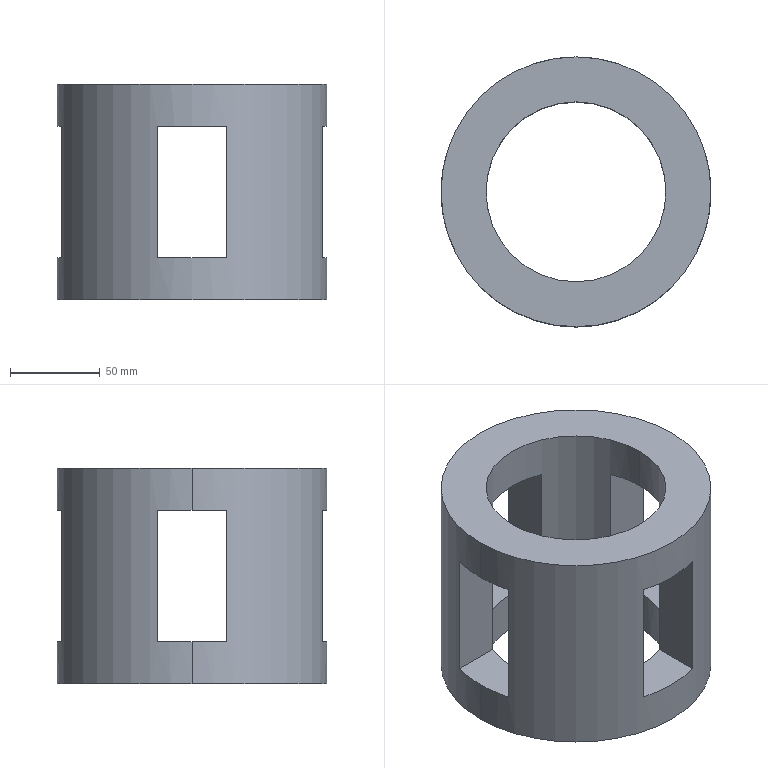Part | SolidWorks | features CirPattern 1, Extrusion 1, ICE 1 | 1 solid | 22 faces | box 150 x 150 x 120 mm | volume 893145 mm3 | plane 18 | cylinder 4 | commonest cylinder face diameters 100 x2 150 x2
STEP:
#1=CARTESIAN_POINT('',(19.196,-46.168,96.484));
#2=VERTEX_POINT('',#1);
#3=CARTESIAN_POINT('',(19.196,-46.168,23.516));
#4=VERTEX_POINT('',#3);
#5=CARTESIAN_POINT('',(19.196,-46.168,120.));
#6=DIRECTION('',(0.,0.,-1.));
#7=VECTOR('',#6,1000.);
#8=LINE('',#5,#7);
#9=EDGE_CURVE('',#2,#4,#8,.T.);
#10=ORIENTED_EDGE('',*,*,#9,.F.);
#11=CARTESIAN_POINT('',(-19.196,-46.168,96.484));
#12=VERTEX_POINT('',#11);
#13=CARTESIAN_POINT('',(0.,0.,96.484));
#14=DIRECTION('',(0.,0.,1.));
#15=DIRECTION('',(1.,0.,0.));
#16=AXIS2_PLACEMENT_3D('',#13,#14,#15);
#17=CIRCLE('',#16,50.);
#18=EDGE_CURVE('',#12,#2,#17,.T.);
#19=ORIENTED_EDGE('',*,*,#18,.F.);
#20=CARTESIAN_POINT('',(-19.196,-46.168,23.516));
#21=VERTEX_POINT('',#20);
#22=CARTESIAN_POINT('',(-19.196,-46.168,120.));
#23=DIRECTION('',(0.,0.,1.));
#24=VECTOR('',#23,1000.);
#25=LINE('',#22,#24);
#26=EDGE_CURVE('',#21,#12,#25,.T.);
#27=ORIENTED_EDGE('',*,*,#26,.F.);
#28=CARTESIAN_POINT('',(0.,0.,23.516));
#29=DIRECTION('',(0.,0.,-1.));
#30=DIRECTION('',(-1.,0.,0.));
#31=AXIS2_PLACEMENT_3D('',#28,#29,#30);
#32=CIRCLE('',#31,50.);
#33=EDGE_CURVE('',#4,#21,#32,.T.);
#34=ORIENTED_EDGE('',*,*,#33,.F.);
#35=EDGE_LOOP('',(#10,#19,#27,#34));
#36=FACE_BOUND('',#35,.T.);
#37=CARTESIAN_POINT('',(-50.,0.,120.));
#38=VERTEX_POINT('',#37);
#39=CARTESIAN_POINT('',(50.,0.,120.));
#40=VERTEX_POINT('',#39);
#41=CARTESIAN_POINT('',(0.,0.,120.));
#42=DIRECTION('',(0.,0.,1.));
#43=DIRECTION('',(1.,0.,0.));
#44=AXIS2_PLACEMENT_3D('',#41,#42,#43);
#45=CIRCLE('',#44,50.);
#46=EDGE_CURVE('',#38,#40,#45,.T.);
#47=ORIENTED_EDGE('',*,*,#46,.T.);
#48=CARTESIAN_POINT('',(50.,0.,96.484));
#49=VERTEX_POINT('',#48);
#50=CARTESIAN_POINT('',(50.,0.,120.));
#51=DIRECTION('',(0.,0.,-1.));
#52=VECTOR('',#51,1000.);
#53=LINE('',#50,#52);
#54=EDGE_CURVE('',#40,#49,#53,.T.);
#55=ORIENTED_EDGE('',*,*,#54,.T.);
#56=CARTESIAN_POINT('',(46.168,-19.196,96.484));
#57=VERTEX_POINT('',#56);
#58=CARTESIAN_POINT('',(0.,0.,96.484));
#59=DIRECTION('',(0.,0.,1.));
#60=DIRECTION('',(1.,0.,0.));
#61=AXIS2_PLACEMENT_3D('',#58,#59,#60);
#62=CIRCLE('',#61,50.);
#63=EDGE_CURVE('',#57,#49,#62,.T.);
#64=ORIENTED_EDGE('',*,*,#63,.F.);
#65=CARTESIAN_POINT('',(46.168,-19.196,23.516));
#66=VERTEX_POINT('',#65);
#67=CARTESIAN_POINT('',(46.168,-19.196,120.));
#68=DIRECTION('',(0.,0.,1.));
#69=VECTOR('',#68,1000.);
#70=LINE('',#67,#69);
#71=EDGE_CURVE('',#66,#57,#70,.T.);
#72=ORIENTED_EDGE('',*,*,#71,.F.);
#73=CARTESIAN_POINT('',(50.,0.,23.516));
#74=VERTEX_POINT('',#73);
#75=CARTESIAN_POINT('',(0.,0.,23.516));
#76=DIRECTION('',(0.,0.,-1.));
#77=DIRECTION('',(-1.,0.,0.));
#78=AXIS2_PLACEMENT_3D('',#75,#76,#77);
#79=CIRCLE('',#78,50.);
#80=EDGE_CURVE('',#74,#66,#79,.T.);
#81=ORIENTED_EDGE('',*,*,#80,.F.);
#82=CARTESIAN_POINT('',(50.,0.,0.));
#83=VERTEX_POINT('',#82);
#84=CARTESIAN_POINT('',(50.,0.,120.));
#85=DIRECTION('',(0.,0.,-1.));
#86=VECTOR('',#85,1000.);
#87=LINE('',#84,#86);
#88=EDGE_CURVE('',#74,#83,#87,.T.);
#89=ORIENTED_EDGE('',*,*,#88,.T.);
#90=CARTESIAN_POINT('',(-50.,0.,0.));
#91=VERTEX_POINT('',#90);
#92=CARTESIAN_POINT('',(0.,0.,0.));
#93=DIRECTION('',(0.,0.,1.));
#94=DIRECTION('',(1.,0.,0.));
#95=AXIS2_PLACEMENT_3D('',#92,#93,#94);
#96=CIRCLE('',#95,50.);
#97=EDGE_CURVE('',#91,#83,#96,.T.);
#98=ORIENTED_EDGE('',*,*,#97,.F.);
#99=CARTESIAN_POINT('',(-50.,0.,23.516));
#100=VERTEX_POINT('',#99);
#101=CARTESIAN_POINT('',(-50.,0.,120.));
#102=DIRECTION('',(0.,0.,-1.));
#103=VECTOR('',#102,1000.);
#104=LINE('',#101,#103);
#105=EDGE_CURVE('',#100,#91,#104,.T.);
#106=ORIENTED_EDGE('',*,*,#105,.F.);
#107=CARTESIAN_POINT('',(-46.168,-19.196,23.516));
#108=VERTEX_POINT('',#107);
#109=CARTESIAN_POINT('',(0.,0.,23.516));
#110=DIRECTION('',(0.,0.,-1.));
#111=DIRECTION('',(-1.,0.,0.));
#112=AXIS2_PLACEMENT_3D('',#109,#110,#111);
#113=CIRCLE('',#112,50.);
#114=EDGE_CURVE('',#108,#100,#113,.T.);
#115=ORIENTED_EDGE('',*,*,#114,.F.);
#116=CARTESIAN_POINT('',(-46.168,-19.196,96.484));
#117=VERTEX_POINT('',#116);
#118=CARTESIAN_POINT('',(-46.168,-19.196,120.));
#119=DIRECTION('',(0.,0.,-1.));
#120=VECTOR('',#119,1000.);
#121=LINE('',#118,#120);
#122=EDGE_CURVE('',#117,#108,#121,.T.);
#123=ORIENTED_EDGE('',*,*,#122,.F.);
#124=CARTESIAN_POINT('',(-50.,0.,96.484));
#125=VERTEX_POINT('',#124);
#126=CARTESIAN_POINT('',(0.,0.,96.484));
#127=DIRECTION('',(0.,0.,1.));
#128=DIRECTION('',(1.,0.,0.));
#129=AXIS2_PLACEMENT_3D('',#126,#127,#128);
#130=CIRCLE('',#129,50.);
#131=EDGE_CURVE('',#125,#117,#130,.T.);
#132=ORIENTED_EDGE('',*,*,#131,.F.);
#133=CARTESIAN_POINT('',(-50.,0.,120.));
#134=DIRECTION('',(0.,0.,-1.));
#135=VECTOR('',#134,1000.);
#136=LINE('',#133,#135);
#137=EDGE_CURVE('',#38,#125,#136,.T.);
#138=ORIENTED_EDGE('',*,*,#137,.F.);
#139=EDGE_LOOP('',(#47,#55,#64,#72,#81,#89,#98,#106,#115,#123,#132,#138));
#140=FACE_OUTER_BOUND('',#139,.T.);
#141=CARTESIAN_POINT('',(0.,0.,120.));
#142=DIRECTION('',(0.,0.,-1.));
#143=DIRECTION('',(-1.,0.,0.));
#144=AXIS2_PLACEMENT_3D('',#141,#142,#143);
#145=CYLINDRICAL_SURFACE('',#144,50.);
#146=ADVANCED_FACE('',(#36,#140),#145,.F.);
#147=CARTESIAN_POINT('',(19.196,72.502,23.516));
#148=VERTEX_POINT('',#147);
#149=CARTESIAN_POINT('',(19.196,72.502,96.484));
#150=VERTEX_POINT('',#149);
#151=CARTESIAN_POINT('',(19.196,72.502,120.));
#152=DIRECTION('',(0.,0.,1.));
#153=VECTOR('',#152,1000.);
#154=LINE('',#151,#153);
#155=EDGE_CURVE('',#148,#150,#154,.T.);
#156=ORIENTED_EDGE('',*,*,#155,.T.);
#157=CARTESIAN_POINT('',(-19.196,72.502,96.484));
#158=VERTEX_POINT('',#157);
#159=CARTESIAN_POINT('',(0.,0.,96.484));
#160=DIRECTION('',(0.,0.,1.));
#161=DIRECTION('',(1.,0.,0.));
#162=AXIS2_PLACEMENT_3D('',#159,#160,#161);
#163=CIRCLE('',#162,75.);
#164=EDGE_CURVE('',#150,#158,#163,.T.);
#165=ORIENTED_EDGE('',*,*,#164,.T.);
#166=CARTESIAN_POINT('',(-19.196,72.502,23.516));
#167=VERTEX_POINT('',#166);
#168=CARTESIAN_POINT('',(-19.196,72.502,120.));
#169=DIRECTION('',(0.,0.,-1.));
#170=VECTOR('',#169,1000.);
#171=LINE('',#168,#170);
#172=EDGE_CURVE('',#158,#167,#171,.T.);
#173=ORIENTED_EDGE('',*,*,#172,.T.);
#174=CARTESIAN_POINT('',(0.,0.,23.516));
#175=DIRECTION('',(0.,0.,-1.));
#176=DIRECTION('',(-1.,0.,0.));
#177=AXIS2_PLACEMENT_3D('',#174,#175,#176);
#178=CIRCLE('',#177,75.);
#179=EDGE_CURVE('',#167,#148,#178,.T.);
#180=ORIENTED_EDGE('',*,*,#179,.T.);
#181=EDGE_LOOP('',(#156,#165,#173,#180));
#182=FACE_BOUND('',#181,.T.);
#183=CARTESIAN_POINT('',(75.,0.,120.));
#184=VERTEX_POINT('',#183);
#185=CARTESIAN_POINT('',(-75.,0.,120.));
#186=VERTEX_POINT('',#185);
#187=CARTESIAN_POINT('',(0.,0.,120.));
#188=DIRECTION('',(0.,0.,1.));
#189=DIRECTION('',(1.,0.,0.));
#190=AXIS2_PLACEMENT_3D('',#187,#188,#189);
#191=CIRCLE('',#190,75.);
#192=EDGE_CURVE('',#184,#186,#191,.T.);
#193=ORIENTED_EDGE('',*,*,#192,.F.);
#194=CARTESIAN_POINT('',(75.,0.,96.484));
#195=VERTEX_POINT('',#194);
#196=CARTESIAN_POINT('',(75.,0.,120.));
#197=DIRECTION('',(0.,0.,-1.));
#198=VECTOR('',#197,1000.);
#199=LINE('',#196,#198);
#200=EDGE_CURVE('',#184,#195,#199,.T.);
#201=ORIENTED_EDGE('',*,*,#200,.T.);
#202=CARTESIAN_POINT('',(72.502,19.196,96.484));
#203=VERTEX_POINT('',#202);
#204=CARTESIAN_POINT('',(0.,0.,96.484));
#205=DIRECTION('',(0.,0.,1.));
#206=DIRECTION('',(1.,0.,0.));
#207=AXIS2_PLACEMENT_3D('',#204,#205,#206);
#208=CIRCLE('',#207,75.);
#209=EDGE_CURVE('',#195,#203,#208,.T.);
#210=ORIENTED_EDGE('',*,*,#209,.T.);
#211=CARTESIAN_POINT('',(72.502,19.196,23.516));
#212=VERTEX_POINT('',#211);
#213=CARTESIAN_POINT('',(72.502,19.196,120.));
#214=DIRECTION('',(0.,0.,-1.));
#215=VECTOR('',#214,1000.);
#216=LINE('',#213,#215);
#217=EDGE_CURVE('',#203,#212,#216,.T.);
#218=ORIENTED_EDGE('',*,*,#217,.T.);
#219=CARTESIAN_POINT('',(75.,0.,23.516));
#220=VERTEX_POINT('',#219);
#221=CARTESIAN_POINT('',(0.,0.,23.516));
#222=DIRECTION('',(0.,0.,-1.));
#223=DIRECTION('',(-1.,0.,0.));
#224=AXIS2_PLACEMENT_3D('',#221,#222,#223);
#225=CIRCLE('',#224,75.);
#226=EDGE_CURVE('',#212,#220,#225,.T.);
#227=ORIENTED_EDGE('',*,*,#226,.T.);
#228=CARTESIAN_POINT('',(75.,0.,0.));
#229=VERTEX_POINT('',#228);
#230=CARTESIAN_POINT('',(75.,0.,120.));
#231=DIRECTION('',(0.,0.,-1.));
#232=VECTOR('',#231,1000.);
#233=LINE('',#230,#232);
#234=EDGE_CURVE('',#220,#229,#233,.T.);
#235=ORIENTED_EDGE('',*,*,#234,.T.);
#236=CARTESIAN_POINT('',(-75.,0.,0.));
#237=VERTEX_POINT('',#236);
#238=CARTESIAN_POINT('',(0.,0.,0.));
#239=DIRECTION('',(0.,0.,1.));
#240=DIRECTION('',(1.,0.,0.));
#241=AXIS2_PLACEMENT_3D('',#238,#239,#240);
#242=CIRCLE('',#241,75.);
#243=EDGE_CURVE('',#229,#237,#242,.T.);
#244=ORIENTED_EDGE('',*,*,#243,.T.);
#245=CARTESIAN_POINT('',(-75.,0.,23.516));
#246=VERTEX_POINT('',#245);
#247=CARTESIAN_POINT('',(-75.,0.,120.));
#248=DIRECTION('',(0.,0.,-1.));
#249=VECTOR('',#248,1000.);
#250=LINE('',#247,#249);
#251=EDGE_CURVE('',#246,#237,#250,.T.);
#252=ORIENTED_EDGE('',*,*,#251,.F.);
#253=CARTESIAN_POINT('',(-72.502,19.196,23.516));
#254=VERTEX_POINT('',#253);
#255=CARTESIAN_POINT('',(0.,0.,23.516));
#256=DIRECTION('',(0.,0.,-1.));
#257=DIRECTION('',(-1.,0.,0.));
#258=AXIS2_PLACEMENT_3D('',#255,#256,#257);
#259=CIRCLE('',#258,75.);
#260=EDGE_CURVE('',#246,#254,#259,.T.);
#261=ORIENTED_EDGE('',*,*,#260,.T.);
#262=CARTESIAN_POINT('',(-72.502,19.196,96.484));
#263=VERTEX_POINT('',#262);
#264=CARTESIAN_POINT('',(-72.502,19.196,120.));
#265=DIRECTION('',(0.,0.,1.));
#266=VECTOR('',#265,1000.);
#267=LINE('',#264,#266);
#268=EDGE_CURVE('',#254,#263,#267,.T.);
#269=ORIENTED_EDGE('',*,*,#268,.T.);
#270=CARTESIAN_POINT('',(-75.,0.,96.484));
#271=VERTEX_POINT('',#270);
#272=CARTESIAN_POINT('',(0.,0.,96.484));
#273=DIRECTION('',(0.,0.,1.));
#274=DIRECTION('',(1.,0.,0.));
#275=AXIS2_PLACEMENT_3D('',#272,#273,#274);
#276=CIRCLE('',#275,75.);
#277=EDGE_CURVE('',#263,#271,#276,.T.);
#278=ORIENTED_EDGE('',*,*,#277,.T.);
#279=CARTESIAN_POINT('',(-75.,0.,120.));
#280=DIRECTION('',(0.,0.,-1.));
#281=VECTOR('',#280,1000.);
#282=LINE('',#279,#281);
#283=EDGE_CURVE('',#186,#271,#282,.T.);
#284=ORIENTED_EDGE('',*,*,#283,.F.);
#285=EDGE_LOOP('',(#193,#201,#210,#218,#227,#235,#244,#252,#261,#269,#278,#284));
#286=FACE_OUTER_BOUND('',#285,.T.);
#287=CARTESIAN_POINT('',(0.,0.,120.));
#288=DIRECTION('',(0.,0.,-1.));
#289=DIRECTION('',(-1.,0.,0.));
#290=AXIS2_PLACEMENT_3D('',#287,#288,#289);
#291=CYLINDRICAL_SURFACE('',#290,75.);
#292=ADVANCED_FACE('',(#182,#286),#291,.T.);
#293=CARTESIAN_POINT('',(0.,0.,120.));
#294=DIRECTION('',(0.,0.,1.));
#295=DIRECTION('',(1.,0.,0.));
#296=AXIS2_PLACEMENT_3D('',#293,#294,#295);
#297=CIRCLE('',#296,75.);
#298=EDGE_CURVE('',#186,#184,#297,.T.);
#299=ORIENTED_EDGE('',*,*,#298,.T.);
#300=ORIENTED_EDGE('',*,*,#192,.T.);
#301=EDGE_LOOP('',(#299,#300));
#302=FACE_OUTER_BOUND('',#301,.T.);
#303=ORIENTED_EDGE('',*,*,#46,.F.);
#304=CARTESIAN_POINT('',(0.,0.,120.));
#305=DIRECTION('',(0.,0.,1.));
#306=DIRECTION('',(1.,0.,0.));
#307=AXIS2_PLACEMENT_3D('',#304,#305,#306);
#308=CIRCLE('',#307,50.);
#309=EDGE_CURVE('',#40,#38,#308,.T.);
#310=ORIENTED_EDGE('',*,*,#309,.F.);
#311=EDGE_LOOP('',(#303,#310));
#312=FACE_BOUND('',#311,.T.);
#313=CARTESIAN_POINT('',(0.,0.,120.));
#314=DIRECTION('',(0.,0.,1.));
#315=DIRECTION('',(1.,0.,0.));
#316=AXIS2_PLACEMENT_3D('',#313,#314,#315);
#317=PLANE('',#316);
#318=ADVANCED_FACE('',(#302,#312),#317,.T.);
#319=CARTESIAN_POINT('',(0.,0.,0.));
#320=DIRECTION('',(0.,0.,1.));
#321=DIRECTION('',(1.,0.,0.));
#322=AXIS2_PLACEMENT_3D('',#319,#320,#321);
#323=CIRCLE('',#322,75.);
#324=EDGE_CURVE('',#237,#229,#323,.T.);
#325=ORIENTED_EDGE('',*,*,#324,.F.);
#326=ORIENTED_EDGE('',*,*,#243,.F.);
#327=EDGE_LOOP('',(#325,#326));
#328=FACE_OUTER_BOUND('',#327,.T.);
#329=ORIENTED_EDGE('',*,*,#97,.T.);
#330=CARTESIAN_POINT('',(0.,0.,0.));
#331=DIRECTION('',(0.,0.,1.));
#332=DIRECTION('',(1.,0.,0.));
#333=AXIS2_PLACEMENT_3D('',#330,#331,#332);
#334=CIRCLE('',#333,50.);
#335=EDGE_CURVE('',#83,#91,#334,.T.);
#336=ORIENTED_EDGE('',*,*,#335,.T.);
#337=EDGE_LOOP('',(#329,#336));
#338=FACE_BOUND('',#337,.T.);
#339=CARTESIAN_POINT('',(0.,0.,0.));
#340=DIRECTION('',(0.,0.,1.));
#341=DIRECTION('',(1.,0.,0.));
#342=AXIS2_PLACEMENT_3D('',#339,#340,#341);
#343=PLANE('',#342);
#344=ADVANCED_FACE('',(#328,#338),#343,.F.);
#345=ORIENTED_EDGE('',*,*,#200,.F.);
#346=ORIENTED_EDGE('',*,*,#298,.F.);
#347=ORIENTED_EDGE('',*,*,#283,.T.);
#348=CARTESIAN_POINT('',(-72.502,-19.196,96.484));
#349=VERTEX_POINT('',#348);
#350=CARTESIAN_POINT('',(0.,0.,96.484));
#351=DIRECTION('',(0.,0.,1.));
#352=DIRECTION('',(1.,0.,0.));
#353=AXIS2_PLACEMENT_3D('',#350,#351,#352);
#354=CIRCLE('',#353,75.);
#355=EDGE_CURVE('',#271,#349,#354,.T.);
#356=ORIENTED_EDGE('',*,*,#355,.T.);
#357=CARTESIAN_POINT('',(-72.502,-19.196,23.516));
#358=VERTEX_POINT('',#357);
#359=CARTESIAN_POINT('',(-72.502,-19.196,120.));
#360=DIRECTION('',(0.,0.,-1.));
#361=VECTOR('',#360,1000.);
#362=LINE('',#359,#361);
#363=EDGE_CURVE('',#349,#358,#362,.T.);
#364=ORIENTED_EDGE('',*,*,#363,.T.);
#365=CARTESIAN_POINT('',(0.,0.,23.516));
#366=DIRECTION('',(0.,0.,-1.));
#367=DIRECTION('',(-1.,0.,0.));
#368=AXIS2_PLACEMENT_3D('',#365,#366,#367);
#369=CIRCLE('',#368,75.);
#370=EDGE_CURVE('',#358,#246,#369,.T.);
#371=ORIENTED_EDGE('',*,*,#370,.T.);
#372=ORIENTED_EDGE('',*,*,#251,.T.);
#373=ORIENTED_EDGE('',*,*,#324,.T.);
#374=ORIENTED_EDGE('',*,*,#234,.F.);
#375=CARTESIAN_POINT('',(72.502,-19.196,23.516));
#376=VERTEX_POINT('',#375);
#377=CARTESIAN_POINT('',(0.,0.,23.516));
#378=DIRECTION('',(0.,0.,-1.));
#379=DIRECTION('',(-1.,0.,0.));
#380=AXIS2_PLACEMENT_3D('',#377,#378,#379);
#381=CIRCLE('',#380,75.);
#382=EDGE_CURVE('',#220,#376,#381,.T.);
#383=ORIENTED_EDGE('',*,*,#382,.T.);
#384=CARTESIAN_POINT('',(72.502,-19.196,96.484));
#385=VERTEX_POINT('',#384);
#386=CARTESIAN_POINT('',(72.502,-19.196,120.));
#387=DIRECTION('',(0.,0.,1.));
#388=VECTOR('',#387,1000.);
#389=LINE('',#386,#388);
#390=EDGE_CURVE('',#376,#385,#389,.T.);
#391=ORIENTED_EDGE('',*,*,#390,.T.);
#392=CARTESIAN_POINT('',(0.,0.,96.484));
#393=DIRECTION('',(0.,0.,1.));
#394=DIRECTION('',(1.,0.,0.));
#395=AXIS2_PLACEMENT_3D('',#392,#393,#394);
#396=CIRCLE('',#395,75.);
#397=EDGE_CURVE('',#385,#195,#396,.T.);
#398=ORIENTED_EDGE('',*,*,#397,.T.);
#399=EDGE_LOOP('',(#345,#346,#347,#356,#364,#371,#372,#373,#374,#383,#391,#398));
#400=FACE_OUTER_BOUND('',#399,.T.);
#401=CARTESIAN_POINT('',(19.196,-72.502,96.484));
#402=VERTEX_POINT('',#401);
#403=CARTESIAN_POINT('',(19.196,-72.502,23.516));
#404=VERTEX_POINT('',#403);
#405=CARTESIAN_POINT('',(19.196,-72.502,120.));
#406=DIRECTION('',(0.,0.,-1.));
#407=VECTOR('',#406,1000.);
#408=LINE('',#405,#407);
#409=EDGE_CURVE('',#402,#404,#408,.T.);
#410=ORIENTED_EDGE('',*,*,#409,.T.);
#411=CARTESIAN_POINT('',(-19.196,-72.502,23.516));
#412=VERTEX_POINT('',#411);
#413=CARTESIAN_POINT('',(0.,0.,23.516));
#414=DIRECTION('',(0.,0.,-1.));
#415=DIRECTION('',(-1.,0.,0.));
#416=AXIS2_PLACEMENT_3D('',#413,#414,#415);
#417=CIRCLE('',#416,75.);
#418=EDGE_CURVE('',#404,#412,#417,.T.);
#419=ORIENTED_EDGE('',*,*,#418,.T.);
#420=CARTESIAN_POINT('',(-19.196,-72.502,96.484));
#421=VERTEX_POINT('',#420);
#422=CARTESIAN_POINT('',(-19.196,-72.502,120.));
#423=DIRECTION('',(0.,0.,1.));
#424=VECTOR('',#423,1000.);
#425=LINE('',#422,#424);
#426=EDGE_CURVE('',#412,#421,#425,.T.);
#427=ORIENTED_EDGE('',*,*,#426,.T.);
#428=CARTESIAN_POINT('',(0.,0.,96.484));
#429=DIRECTION('',(0.,0.,1.));
#430=DIRECTION('',(1.,0.,0.));
#431=AXIS2_PLACEMENT_3D('',#428,#429,#430);
#432=CIRCLE('',#431,75.);
#433=EDGE_CURVE('',#421,#402,#432,.T.);
#434=ORIENTED_EDGE('',*,*,#433,.T.);
#435=EDGE_LOOP('',(#410,#419,#427,#434));
#436=FACE_BOUND('',#435,.T.);
#437=CARTESIAN_POINT('',(0.,0.,120.));
#438=DIRECTION('',(0.,0.,-1.));
#439=DIRECTION('',(-1.,0.,0.));
#440=AXIS2_PLACEMENT_3D('',#437,#438,#439);
#441=CYLINDRICAL_SURFACE('',#440,75.);
#442=ADVANCED_FACE('',(#400,#436),#441,.T.);
#443=ORIENTED_EDGE('',*,*,#54,.F.);
#444=ORIENTED_EDGE('',*,*,#309,.T.);
#445=ORIENTED_EDGE('',*,*,#137,.T.);
#446=CARTESIAN_POINT('',(-46.168,19.196,96.484));
#447=VERTEX_POINT('',#446);
#448=CARTESIAN_POINT('',(0.,0.,96.484));
#449=DIRECTION('',(0.,0.,1.));
#450=DIRECTION('',(1.,0.,0.));
#451=AXIS2_PLACEMENT_3D('',#448,#449,#450);
#452=CIRCLE('',#451,50.);
#453=EDGE_CURVE('',#447,#125,#452,.T.);
#454=ORIENTED_EDGE('',*,*,#453,.F.);
#455=CARTESIAN_POINT('',(-46.168,19.196,23.516));
#456=VERTEX_POINT('',#455);
#457=CARTESIAN_POINT('',(-46.168,19.196,120.));
#458=DIRECTION('',(0.,0.,1.));
#459=VECTOR('',#458,1000.);
#460=LINE('',#457,#459);
#461=EDGE_CURVE('',#456,#447,#460,.T.);
#462=ORIENTED_EDGE('',*,*,#461,.F.);
#463=CARTESIAN_POINT('',(0.,0.,23.516));
#464=DIRECTION('',(0.,0.,-1.));
#465=DIRECTION('',(-1.,0.,0.));
#466=AXIS2_PLACEMENT_3D('',#463,#464,#465);
#467=CIRCLE('',#466,50.);
#468=EDGE_CURVE('',#100,#456,#467,.T.);
#469=ORIENTED_EDGE('',*,*,#468,.F.);
#470=ORIENTED_EDGE('',*,*,#105,.T.);
#471=ORIENTED_EDGE('',*,*,#335,.F.);
#472=ORIENTED_EDGE('',*,*,#88,.F.);
#473=CARTESIAN_POINT('',(46.168,19.196,23.516));
#474=VERTEX_POINT('',#473);
#475=CARTESIAN_POINT('',(0.,0.,23.516));
#476=DIRECTION('',(0.,0.,-1.));
#477=DIRECTION('',(-1.,0.,0.));
#478=AXIS2_PLACEMENT_3D('',#475,#476,#477);
#479=CIRCLE('',#478,50.);
#480=EDGE_CURVE('',#474,#74,#479,.T.);
#481=ORIENTED_EDGE('',*,*,#480,.F.);
#482=CARTESIAN_POINT('',(46.168,19.196,96.484));
#483=VERTEX_POINT('',#482);
#484=CARTESIAN_POINT('',(46.168,19.196,120.));
#485=DIRECTION('',(0.,0.,-1.));
#486=VECTOR('',#485,1000.);
#487=LINE('',#484,#486);
#488=EDGE_CURVE('',#483,#474,#487,.T.);
#489=ORIENTED_EDGE('',*,*,#488,.F.);
#490=CARTESIAN_POINT('',(0.,0.,96.484));
#491=DIRECTION('',(0.,0.,1.));
#492=DIRECTION('',(1.,0.,0.));
#493=AXIS2_PLACEMENT_3D('',#490,#491,#492);
#494=CIRCLE('',#493,50.);
#495=EDGE_CURVE('',#49,#483,#494,.T.);
#496=ORIENTED_EDGE('',*,*,#495,.F.);
#497=EDGE_LOOP('',(#443,#444,#445,#454,#462,#469,#470,#471,#472,#481,#489,#496));
#498=FACE_OUTER_BOUND('',#497,.T.);
#499=CARTESIAN_POINT('',(-19.196,46.168,96.484));
#500=VERTEX_POINT('',#499);
#501=CARTESIAN_POINT('',(-19.196,46.168,23.516));
#502=VERTEX_POINT('',#501);
#503=CARTESIAN_POINT('',(-19.196,46.168,120.));
#504=DIRECTION('',(0.,0.,-1.));
#505=VECTOR('',#504,1000.);
#506=LINE('',#503,#505);
#507=EDGE_CURVE('',#500,#502,#506,.T.);
#508=ORIENTED_EDGE('',*,*,#507,.F.);
#509=CARTESIAN_POINT('',(19.196,46.168,96.484));
#510=VERTEX_POINT('',#509);
#511=CARTESIAN_POINT('',(0.,0.,96.484));
#512=DIRECTION('',(0.,0.,1.));
#513=DIRECTION('',(1.,0.,0.));
#514=AXIS2_PLACEMENT_3D('',#511,#512,#513);
#515=CIRCLE('',#514,50.);
#516=EDGE_CURVE('',#510,#500,#515,.T.);
#517=ORIENTED_EDGE('',*,*,#516,.F.);
#518=CARTESIAN_POINT('',(19.196,46.168,23.516));
#519=VERTEX_POINT('',#518);
#520=CARTESIAN_POINT('',(19.196,46.168,120.));
#521=DIRECTION('',(0.,0.,1.));
#522=VECTOR('',#521,1000.);
#523=LINE('',#520,#522);
#524=EDGE_CURVE('',#519,#510,#523,.T.);
#525=ORIENTED_EDGE('',*,*,#524,.F.);
#526=CARTESIAN_POINT('',(0.,0.,23.516));
#527=DIRECTION('',(0.,0.,-1.));
#528=DIRECTION('',(-1.,0.,0.));
#529=AXIS2_PLACEMENT_3D('',#526,#527,#528);
#530=CIRCLE('',#529,50.);
#531=EDGE_CURVE('',#502,#519,#530,.T.);
#532=ORIENTED_EDGE('',*,*,#531,.F.);
#533=EDGE_LOOP('',(#508,#517,#525,#532));
#534=FACE_BOUND('',#533,.T.);
#535=CARTESIAN_POINT('',(0.,0.,120.));
#536=DIRECTION('',(0.,0.,-1.));
#537=DIRECTION('',(-1.,0.,0.));
#538=AXIS2_PLACEMENT_3D('',#535,#536,#537);
#539=CYLINDRICAL_SURFACE('',#538,50.);
#540=ADVANCED_FACE('',(#498,#534),#539,.F.);
#541=CARTESIAN_POINT('',(19.196,-75.,96.484));
#542=DIRECTION('',(0.,1.,0.));
#543=VECTOR('',#542,1000.);
#544=LINE('',#541,#543);
#545=EDGE_CURVE('',#402,#2,#544,.T.);
#546=ORIENTED_EDGE('',*,*,#545,.T.);
#547=ORIENTED_EDGE('',*,*,#9,.T.);
#548=CARTESIAN_POINT('',(19.196,-75.,23.516));
#549=DIRECTION('',(0.,1.,0.));
#550=VECTOR('',#549,1000.);
#551=LINE('',#548,#550);
#552=EDGE_CURVE('',#404,#4,#551,.T.);
#553=ORIENTED_EDGE('',*,*,#552,.F.);
#554=ORIENTED_EDGE('',*,*,#409,.F.);
#555=EDGE_LOOP('',(#546,#547,#553,#554));
#556=FACE_OUTER_BOUND('',#555,.T.);
#557=CARTESIAN_POINT('',(19.196,-75.,23.516));
#558=DIRECTION('',(1.,0.,0.));
#559=DIRECTION('',(0.,0.,-1.));
#560=AXIS2_PLACEMENT_3D('',#557,#558,#559);
#561=PLANE('',#560);
#562=ADVANCED_FACE('',(#556),#561,.F.);
#563=CARTESIAN_POINT('',(-19.196,-75.,96.484));
#564=DIRECTION('',(0.,1.,0.));
#565=VECTOR('',#564,1000.);
#566=LINE('',#563,#565);
#567=EDGE_CURVE('',#421,#12,#566,.T.);
#568=ORIENTED_EDGE('',*,*,#567,.T.);
#569=ORIENTED_EDGE('',*,*,#18,.T.);
#570=ORIENTED_EDGE('',*,*,#545,.F.);
#571=ORIENTED_EDGE('',*,*,#433,.F.);
#572=EDGE_LOOP('',(#568,#569,#570,#571));
#573=FACE_OUTER_BOUND('',#572,.T.);
#574=CARTESIAN_POINT('',(-19.196,-75.,96.484));
#575=DIRECTION('',(0.,0.,1.));
#576=DIRECTION('',(1.,0.,0.));
#577=AXIS2_PLACEMENT_3D('',#574,#575,#576);
#578=PLANE('',#577);
#579=ADVANCED_FACE('',(#573),#578,.F.);
#580=CARTESIAN_POINT('',(-19.196,-75.,23.516));
#581=DIRECTION('',(0.,1.,0.));
#582=VECTOR('',#581,1000.);
#583=LINE('',#580,#582);
#584=EDGE_CURVE('',#412,#21,#583,.T.);
#585=ORIENTED_EDGE('',*,*,#584,.T.);
#586=ORIENTED_EDGE('',*,*,#26,.T.);
#587=ORIENTED_EDGE('',*,*,#567,.F.);
#588=ORIENTED_EDGE('',*,*,#426,.F.);
#589=EDGE_LOOP('',(#585,#586,#587,#588));
#590=FACE_OUTER_BOUND('',#589,.T.);
#591=CARTESIAN_POINT('',(-19.196,-75.,23.516));
#592=DIRECTION('',(-1.,0.,0.));
#593=DIRECTION('',(0.,0.,1.));
#594=AXIS2_PLACEMENT_3D('',#591,#592,#593);
#595=PLANE('',#594);
#596=ADVANCED_FACE('',(#590),#595,.F.);
#597=ORIENTED_EDGE('',*,*,#552,.T.);
#598=ORIENTED_EDGE('',*,*,#33,.T.);
#599=ORIENTED_EDGE('',*,*,#584,.F.);
#600=ORIENTED_EDGE('',*,*,#418,.F.);
#601=EDGE_LOOP('',(#597,#598,#599,#600));
#602=FACE_OUTER_BOUND('',#601,.T.);
#603=CARTESIAN_POINT('',(-19.196,-75.,23.516));
#604=DIRECTION('',(0.,0.,-1.));
#605=DIRECTION('',(-1.,0.,0.));
#606=AXIS2_PLACEMENT_3D('',#603,#604,#605);
#607=PLANE('',#606);
#608=ADVANCED_FACE('',(#602),#607,.F.);
#609=CARTESIAN_POINT('',(75.,19.196,96.484));
#610=DIRECTION('',(-1.,0.,0.));
#611=VECTOR('',#610,1000.);
#612=LINE('',#609,#611);
#613=EDGE_CURVE('',#203,#483,#612,.T.);
#614=ORIENTED_EDGE('',*,*,#613,.T.);
#615=ORIENTED_EDGE('',*,*,#488,.T.);
#616=CARTESIAN_POINT('',(75.,19.196,23.516));
#617=DIRECTION('',(-1.,0.,0.));
#618=VECTOR('',#617,1000.);
#619=LINE('',#616,#618);
#620=EDGE_CURVE('',#212,#474,#619,.T.);
#621=ORIENTED_EDGE('',*,*,#620,.F.);
#622=ORIENTED_EDGE('',*,*,#217,.F.);
#623=EDGE_LOOP('',(#614,#615,#621,#622));
#624=FACE_OUTER_BOUND('',#623,.T.);
#625=CARTESIAN_POINT('',(75.,19.196,23.516));
#626=DIRECTION('',(0.,1.,0.));
#627=DIRECTION('',(-1.,0.,0.));
#628=AXIS2_PLACEMENT_3D('',#625,#626,#627);
#629=PLANE('',#628);
#630=ADVANCED_FACE('',(#624),#629,.F.);
#631=ORIENTED_EDGE('',*,*,#620,.T.);
#632=ORIENTED_EDGE('',*,*,#480,.T.);
#633=ORIENTED_EDGE('',*,*,#80,.T.);
#634=CARTESIAN_POINT('',(-75.,-19.196,23.516));
#635=DIRECTION('',(1.,0.,0.));
#636=VECTOR('',#635,1000.);
#637=LINE('',#634,#636);
#638=EDGE_CURVE('',#66,#376,#637,.T.);
#639=ORIENTED_EDGE('',*,*,#638,.T.);
#640=ORIENTED_EDGE('',*,*,#382,.F.);
#641=ORIENTED_EDGE('',*,*,#226,.F.);
#642=EDGE_LOOP('',(#631,#632,#633,#639,#640,#641));
#643=FACE_OUTER_BOUND('',#642,.T.);
#644=CARTESIAN_POINT('',(-75.,19.196,23.516));
#645=DIRECTION('',(0.,0.,-1.));
#646=DIRECTION('',(-1.,0.,0.));
#647=AXIS2_PLACEMENT_3D('',#644,#645,#646);
#648=PLANE('',#647);
#649=ADVANCED_FACE('',(#643),#648,.F.);
#650=ORIENTED_EDGE('',*,*,#397,.F.);
#651=CARTESIAN_POINT('',(-75.,-19.196,96.484));
#652=DIRECTION('',(1.,0.,0.));
#653=VECTOR('',#652,1000.);
#654=LINE('',#651,#653);
#655=EDGE_CURVE('',#57,#385,#654,.T.);
#656=ORIENTED_EDGE('',*,*,#655,.F.);
#657=ORIENTED_EDGE('',*,*,#63,.T.);
#658=ORIENTED_EDGE('',*,*,#495,.T.);
#659=ORIENTED_EDGE('',*,*,#613,.F.);
#660=ORIENTED_EDGE('',*,*,#209,.F.);
#661=EDGE_LOOP('',(#650,#656,#657,#658,#659,#660));
#662=FACE_OUTER_BOUND('',#661,.T.);
#663=CARTESIAN_POINT('',(-75.,19.196,96.484));
#664=DIRECTION('',(0.,0.,1.));
#665=DIRECTION('',(1.,0.,0.));
#666=AXIS2_PLACEMENT_3D('',#663,#664,#665);
#667=PLANE('',#666);
#668=ADVANCED_FACE('',(#662),#667,.F.);
#669=ORIENTED_EDGE('',*,*,#638,.F.);
#670=ORIENTED_EDGE('',*,*,#71,.T.);
#671=ORIENTED_EDGE('',*,*,#655,.T.);
#672=ORIENTED_EDGE('',*,*,#390,.F.);
#673=EDGE_LOOP('',(#669,#670,#671,#672));
#674=FACE_OUTER_BOUND('',#673,.T.);
#675=CARTESIAN_POINT('',(-75.,-19.196,23.516));
#676=DIRECTION('',(0.,-1.,0.));
#677=DIRECTION('',(1.,0.,0.));
#678=AXIS2_PLACEMENT_3D('',#675,#676,#677);
#679=PLANE('',#678);
#680=ADVANCED_FACE('',(#674),#679,.F.);
#681=CARTESIAN_POINT('',(19.196,75.,23.516));
#682=DIRECTION('',(0.,-1.,0.));
#683=VECTOR('',#682,1000.);
#684=LINE('',#681,#683);
#685=EDGE_CURVE('',#148,#519,#684,.T.);
#686=ORIENTED_EDGE('',*,*,#685,.T.);
#687=ORIENTED_EDGE('',*,*,#524,.T.);
#688=CARTESIAN_POINT('',(19.196,75.,96.484));
#689=DIRECTION('',(0.,-1.,0.));
#690=VECTOR('',#689,1000.);
#691=LINE('',#688,#690);
#692=EDGE_CURVE('',#150,#510,#691,.T.);
#693=ORIENTED_EDGE('',*,*,#692,.F.);
#694=ORIENTED_EDGE('',*,*,#155,.F.);
#695=EDGE_LOOP('',(#686,#687,#693,#694));
#696=FACE_OUTER_BOUND('',#695,.T.);
#697=CARTESIAN_POINT('',(19.196,75.,23.516));
#698=DIRECTION('',(1.,0.,0.));
#699=DIRECTION('',(0.,0.,-1.));
#700=AXIS2_PLACEMENT_3D('',#697,#698,#699);
#701=PLANE('',#700);
#702=ADVANCED_FACE('',(#696),#701,.F.);
#703=CARTESIAN_POINT('',(-19.196,75.,96.484));
#704=DIRECTION('',(0.,-1.,0.));
#705=VECTOR('',#704,1000.);
#706=LINE('',#703,#705);
#707=EDGE_CURVE('',#158,#500,#706,.T.);
#708=ORIENTED_EDGE('',*,*,#707,.T.);
#709=ORIENTED_EDGE('',*,*,#507,.T.);
#710=CARTESIAN_POINT('',(-19.196,75.,23.516));
#711=DIRECTION('',(0.,-1.,0.));
#712=VECTOR('',#711,1000.);
#713=LINE('',#710,#712);
#714=EDGE_CURVE('',#167,#502,#713,.T.);
#715=ORIENTED_EDGE('',*,*,#714,.F.);
#716=ORIENTED_EDGE('',*,*,#172,.F.);
#717=EDGE_LOOP('',(#708,#709,#715,#716));
#718=FACE_OUTER_BOUND('',#717,.T.);
#719=CARTESIAN_POINT('',(-19.196,75.,23.516));
#720=DIRECTION('',(-1.,0.,0.));
#721=DIRECTION('',(0.,0.,1.));
#722=AXIS2_PLACEMENT_3D('',#719,#720,#721);
#723=PLANE('',#722);
#724=ADVANCED_FACE('',(#718),#723,.F.);
#725=ORIENTED_EDGE('',*,*,#714,.T.);
#726=ORIENTED_EDGE('',*,*,#531,.T.);
#727=ORIENTED_EDGE('',*,*,#685,.F.);
#728=ORIENTED_EDGE('',*,*,#179,.F.);
#729=EDGE_LOOP('',(#725,#726,#727,#728));
#730=FACE_OUTER_BOUND('',#729,.T.);
#731=CARTESIAN_POINT('',(-75.,19.196,23.516));
#732=DIRECTION('',(0.,0.,-1.));
#733=DIRECTION('',(-1.,0.,0.));
#734=AXIS2_PLACEMENT_3D('',#731,#732,#733);
#735=PLANE('',#734);
#736=ADVANCED_FACE('',(#730),#735,.F.);
#737=ORIENTED_EDGE('',*,*,#692,.T.);
#738=ORIENTED_EDGE('',*,*,#516,.T.);
#739=ORIENTED_EDGE('',*,*,#707,.F.);
#740=ORIENTED_EDGE('',*,*,#164,.F.);
#741=EDGE_LOOP('',(#737,#738,#739,#740));
#742=FACE_OUTER_BOUND('',#741,.T.);
#743=CARTESIAN_POINT('',(-75.,19.196,96.484));
#744=DIRECTION('',(0.,0.,1.));
#745=DIRECTION('',(1.,0.,0.));
#746=AXIS2_PLACEMENT_3D('',#743,#744,#745);
#747=PLANE('',#746);
#748=ADVANCED_FACE('',(#742),#747,.F.);
#749=CARTESIAN_POINT('',(-75.,-19.196,96.484));
#750=DIRECTION('',(1.,0.,0.));
#751=VECTOR('',#750,1000.);
#752=LINE('',#749,#751);
#753=EDGE_CURVE('',#349,#117,#752,.T.);
#754=ORIENTED_EDGE('',*,*,#753,.T.);
#755=ORIENTED_EDGE('',*,*,#122,.T.);
#756=CARTESIAN_POINT('',(-75.,-19.196,23.516));
#757=DIRECTION('',(1.,0.,0.));
#758=VECTOR('',#757,1000.);
#759=LINE('',#756,#758);
#760=EDGE_CURVE('',#358,#108,#759,.T.);
#761=ORIENTED_EDGE('',*,*,#760,.F.);
#762=ORIENTED_EDGE('',*,*,#363,.F.);
#763=EDGE_LOOP('',(#754,#755,#761,#762));
#764=FACE_OUTER_BOUND('',#763,.T.);
#765=CARTESIAN_POINT('',(-75.,-19.196,23.516));
#766=DIRECTION('',(0.,-1.,0.));
#767=DIRECTION('',(1.,0.,0.));
#768=AXIS2_PLACEMENT_3D('',#765,#766,#767);
#769=PLANE('',#768);
#770=ADVANCED_FACE('',(#764),#769,.F.);
#771=CARTESIAN_POINT('',(-75.,19.196,96.484));
#772=DIRECTION('',(1.,0.,0.));
#773=VECTOR('',#772,1000.);
#774=LINE('',#771,#773);
#775=EDGE_CURVE('',#263,#447,#774,.T.);
#776=ORIENTED_EDGE('',*,*,#775,.T.);
#777=ORIENTED_EDGE('',*,*,#453,.T.);
#778=ORIENTED_EDGE('',*,*,#131,.T.);
#779=ORIENTED_EDGE('',*,*,#753,.F.);
#780=ORIENTED_EDGE('',*,*,#355,.F.);
#781=ORIENTED_EDGE('',*,*,#277,.F.);
#782=EDGE_LOOP('',(#776,#777,#778,#779,#780,#781));
#783=FACE_OUTER_BOUND('',#782,.T.);
#784=CARTESIAN_POINT('',(-75.,19.196,96.484));
#785=DIRECTION('',(0.,0.,1.));
#786=DIRECTION('',(1.,0.,0.));
#787=AXIS2_PLACEMENT_3D('',#784,#785,#786);
#788=PLANE('',#787);
#789=ADVANCED_FACE('',(#783),#788,.F.);
#790=CARTESIAN_POINT('',(-75.,19.196,23.516));
#791=DIRECTION('',(1.,0.,0.));
#792=VECTOR('',#791,1000.);
#793=LINE('',#790,#792);
#794=EDGE_CURVE('',#254,#456,#793,.T.);
#795=ORIENTED_EDGE('',*,*,#794,.T.);
#796=ORIENTED_EDGE('',*,*,#461,.T.);
#797=ORIENTED_EDGE('',*,*,#775,.F.);
#798=ORIENTED_EDGE('',*,*,#268,.F.);
#799=EDGE_LOOP('',(#795,#796,#797,#798));
#800=FACE_OUTER_BOUND('',#799,.T.);
#801=CARTESIAN_POINT('',(-75.,19.196,23.516));
#802=DIRECTION('',(0.,1.,0.));
#803=DIRECTION('',(-1.,0.,0.));
#804=AXIS2_PLACEMENT_3D('',#801,#802,#803);
#805=PLANE('',#804);
#806=ADVANCED_FACE('',(#800),#805,.F.);
#807=ORIENTED_EDGE('',*,*,#370,.F.);
#808=ORIENTED_EDGE('',*,*,#760,.T.);
#809=ORIENTED_EDGE('',*,*,#114,.T.);
#810=ORIENTED_EDGE('',*,*,#468,.T.);
#811=ORIENTED_EDGE('',*,*,#794,.F.);
#812=ORIENTED_EDGE('',*,*,#260,.F.);
#813=EDGE_LOOP('',(#807,#808,#809,#810,#811,#812));
#814=FACE_OUTER_BOUND('',#813,.T.);
#815=CARTESIAN_POINT('',(-75.,19.196,23.516));
#816=DIRECTION('',(0.,0.,-1.));
#817=DIRECTION('',(-1.,0.,0.));
#818=AXIS2_PLACEMENT_3D('',#815,#816,#817);
#819=PLANE('',#818);
#820=ADVANCED_FACE('',(#814),#819,.F.);
#821=CLOSED_SHELL('',(#146,#292,#318,#344,#442,#540,#562,#579,#596,#608,#630,#649,#668,#680,#702,#724,#736,#748,#770,#789,#806,#820));
#822=MANIFOLD_SOLID_BREP('',#821);
#823=CARTESIAN_POINT('',(0.,0.,0.));
#824=DIRECTION('',(0.,0.,1.));
#825=DIRECTION('',(1.,0.,0.));
#826=AXIS2_PLACEMENT_3D('',#823,#824,#825);
#827=(LENGTH_UNIT()NAMED_UNIT(*)SI_UNIT(.MILLI.,.METRE.));
#828=UNCERTAINTY_MEASURE_WITH_UNIT(LENGTH_MEASURE(0.00001),#827,'','');
#829=(NAMED_UNIT(*)PLANE_ANGLE_UNIT()SI_UNIT($,.RADIAN.));
#830=(NAMED_UNIT(*)SI_UNIT($,.STERADIAN.)SOLID_ANGLE_UNIT());
#831=(GEOMETRIC_REPRESENTATION_CONTEXT(3)GLOBAL_UNCERTAINTY_ASSIGNED_CONTEXT((#828))GLOBAL_UNIT_ASSIGNED_CONTEXT((#827,#829,#830))REPRESENTATION_CONTEXT('',''));
#832=ADVANCED_BREP_SHAPE_REPRESENTATION('',(#822,#826),#831);